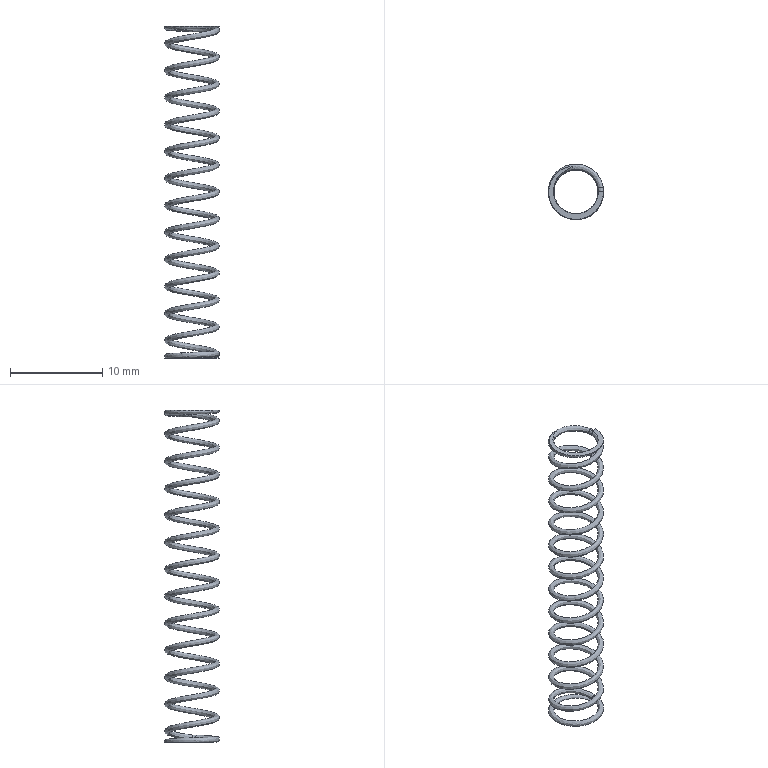Part | STEP file | 200 mesh_id1686 | 1 solid | 9 faces | volume 65.446 mm3 | spline 5 | plane 4